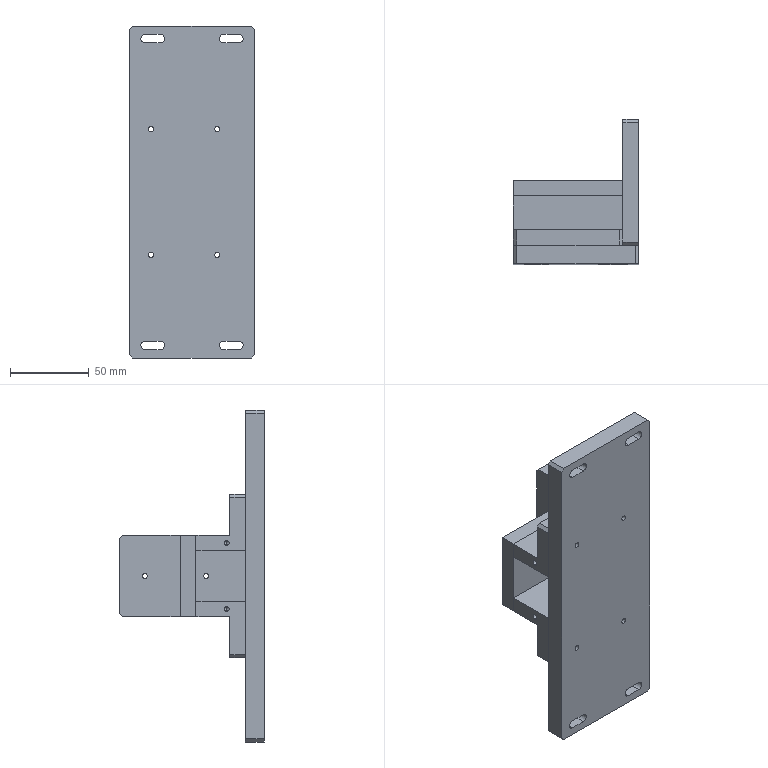Part | STEP file | 1105-104P044 | 5 solids | 230 faces | box 79.5 x 92 x 211 mm | volume 345527 mm3 | cylinder 112 | plane 94 | cone 24 | commonest cylinder face diameters 3.3 x32 4.5 x28 8 x28 5.5 x8 10 x8 4 x4